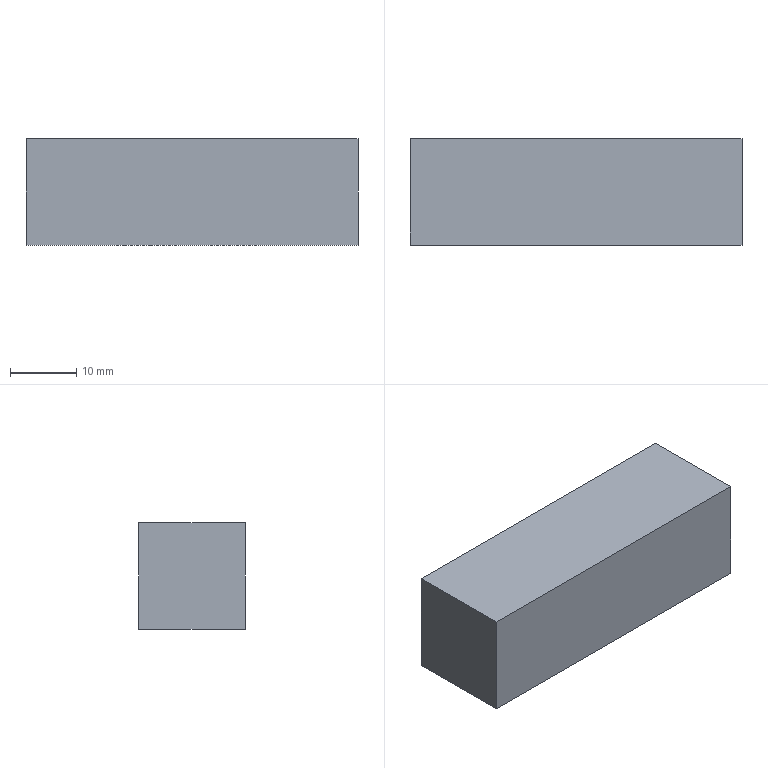Part | STEP file | [21]-1 | 1 solid | 6 faces | box 50 x 16 x 16 mm | volume 12800 mm3 | plane 6
STEP:
#1=CARTESIAN_POINT('',(0.,0.,0.));
#2=VERTEX_POINT('',#1);
#3=CARTESIAN_POINT('',(0.,16.,0.));
#4=VERTEX_POINT('',#3);
#5=CARTESIAN_POINT('',(0.,8.,0.));
#6=DIRECTION('',(0.,1.,0.));
#7=VECTOR('',#6,1000.);
#8=LINE('',#5,#7);
#9=EDGE_CURVE('',#2,#4,#8,.T.);
#10=ORIENTED_EDGE('',*,*,#9,.F.);
#11=CARTESIAN_POINT('',(0.,0.,16.));
#12=VERTEX_POINT('',#11);
#13=CARTESIAN_POINT('',(0.,0.,8.));
#14=DIRECTION('',(0.,0.,-1.));
#15=VECTOR('',#14,1000.);
#16=LINE('',#13,#15);
#17=EDGE_CURVE('',#12,#2,#16,.T.);
#18=ORIENTED_EDGE('',*,*,#17,.F.);
#19=CARTESIAN_POINT('',(0.,16.,16.));
#20=VERTEX_POINT('',#19);
#21=CARTESIAN_POINT('',(0.,8.,16.));
#22=DIRECTION('',(0.,-1.,0.));
#23=VECTOR('',#22,1000.);
#24=LINE('',#21,#23);
#25=EDGE_CURVE('',#20,#12,#24,.T.);
#26=ORIENTED_EDGE('',*,*,#25,.F.);
#27=CARTESIAN_POINT('',(0.,16.,8.));
#28=DIRECTION('',(0.,0.,1.));
#29=VECTOR('',#28,1000.);
#30=LINE('',#27,#29);
#31=EDGE_CURVE('',#4,#20,#30,.T.);
#32=ORIENTED_EDGE('',*,*,#31,.F.);
#33=EDGE_LOOP('',(#10,#18,#26,#32));
#34=FACE_OUTER_BOUND('',#33,.T.);
#35=CARTESIAN_POINT('',(0.,8.,8.));
#36=DIRECTION('',(-1.,0.,0.));
#37=DIRECTION('',(0.,-1.,0.));
#38=AXIS2_PLACEMENT_3D('',#35,#36,#37);
#39=PLANE('',#38);
#40=ADVANCED_FACE('',(#34),#39,.T.);
#41=CARTESIAN_POINT('',(50.,0.,0.));
#42=VERTEX_POINT('',#41);
#43=CARTESIAN_POINT('',(50.,0.,0.));
#44=DIRECTION('',(-1.,0.,0.));
#45=VECTOR('',#44,1000.);
#46=LINE('',#43,#45);
#47=EDGE_CURVE('',#42,#2,#46,.T.);
#48=ORIENTED_EDGE('',*,*,#47,.T.);
#49=ORIENTED_EDGE('',*,*,#9,.T.);
#50=CARTESIAN_POINT('',(50.,16.,0.));
#51=VERTEX_POINT('',#50);
#52=CARTESIAN_POINT('',(50.,16.,0.));
#53=DIRECTION('',(-1.,0.,0.));
#54=VECTOR('',#53,1000.);
#55=LINE('',#52,#54);
#56=EDGE_CURVE('',#51,#4,#55,.T.);
#57=ORIENTED_EDGE('',*,*,#56,.F.);
#58=CARTESIAN_POINT('',(50.,8.,0.));
#59=DIRECTION('',(0.,-1.,0.));
#60=VECTOR('',#59,1000.);
#61=LINE('',#58,#60);
#62=EDGE_CURVE('',#51,#42,#61,.T.);
#63=ORIENTED_EDGE('',*,*,#62,.T.);
#64=EDGE_LOOP('',(#48,#49,#57,#63));
#65=FACE_OUTER_BOUND('',#64,.T.);
#66=CARTESIAN_POINT('',(50.,8.,0.));
#67=DIRECTION('',(0.,0.,-1.));
#68=DIRECTION('',(1.,0.,0.));
#69=AXIS2_PLACEMENT_3D('',#66,#67,#68);
#70=PLANE('',#69);
#71=ADVANCED_FACE('',(#65),#70,.T.);
#72=ORIENTED_EDGE('',*,*,#56,.T.);
#73=ORIENTED_EDGE('',*,*,#31,.T.);
#74=CARTESIAN_POINT('',(50.,16.,16.));
#75=VERTEX_POINT('',#74);
#76=CARTESIAN_POINT('',(50.,16.,16.));
#77=DIRECTION('',(-1.,0.,0.));
#78=VECTOR('',#77,1000.);
#79=LINE('',#76,#78);
#80=EDGE_CURVE('',#75,#20,#79,.T.);
#81=ORIENTED_EDGE('',*,*,#80,.F.);
#82=CARTESIAN_POINT('',(50.,16.,8.));
#83=DIRECTION('',(0.,0.,-1.));
#84=VECTOR('',#83,1000.);
#85=LINE('',#82,#84);
#86=EDGE_CURVE('',#75,#51,#85,.T.);
#87=ORIENTED_EDGE('',*,*,#86,.T.);
#88=EDGE_LOOP('',(#72,#73,#81,#87));
#89=FACE_OUTER_BOUND('',#88,.T.);
#90=CARTESIAN_POINT('',(50.,16.,8.));
#91=DIRECTION('',(0.,1.,0.));
#92=DIRECTION('',(-1.,0.,0.));
#93=AXIS2_PLACEMENT_3D('',#90,#91,#92);
#94=PLANE('',#93);
#95=ADVANCED_FACE('',(#89),#94,.T.);
#96=ORIENTED_EDGE('',*,*,#80,.T.);
#97=ORIENTED_EDGE('',*,*,#25,.T.);
#98=CARTESIAN_POINT('',(50.,0.,16.));
#99=VERTEX_POINT('',#98);
#100=CARTESIAN_POINT('',(50.,0.,16.));
#101=DIRECTION('',(-1.,0.,0.));
#102=VECTOR('',#101,1000.);
#103=LINE('',#100,#102);
#104=EDGE_CURVE('',#99,#12,#103,.T.);
#105=ORIENTED_EDGE('',*,*,#104,.F.);
#106=CARTESIAN_POINT('',(50.,8.,16.));
#107=DIRECTION('',(0.,1.,0.));
#108=VECTOR('',#107,1000.);
#109=LINE('',#106,#108);
#110=EDGE_CURVE('',#99,#75,#109,.T.);
#111=ORIENTED_EDGE('',*,*,#110,.T.);
#112=EDGE_LOOP('',(#96,#97,#105,#111));
#113=FACE_OUTER_BOUND('',#112,.T.);
#114=CARTESIAN_POINT('',(50.,8.,16.));
#115=DIRECTION('',(0.,0.,1.));
#116=DIRECTION('',(-1.,0.,0.));
#117=AXIS2_PLACEMENT_3D('',#114,#115,#116);
#118=PLANE('',#117);
#119=ADVANCED_FACE('',(#113),#118,.T.);
#120=CARTESIAN_POINT('',(50.,0.,8.));
#121=DIRECTION('',(0.,0.,1.));
#122=VECTOR('',#121,1000.);
#123=LINE('',#120,#122);
#124=EDGE_CURVE('',#42,#99,#123,.T.);
#125=ORIENTED_EDGE('',*,*,#124,.F.);
#126=ORIENTED_EDGE('',*,*,#62,.F.);
#127=ORIENTED_EDGE('',*,*,#86,.F.);
#128=ORIENTED_EDGE('',*,*,#110,.F.);
#129=EDGE_LOOP('',(#125,#126,#127,#128));
#130=FACE_OUTER_BOUND('',#129,.T.);
#131=CARTESIAN_POINT('',(50.,8.,8.));
#132=DIRECTION('',(1.,0.,0.));
#133=DIRECTION('',(0.,1.,0.));
#134=AXIS2_PLACEMENT_3D('',#131,#132,#133);
#135=PLANE('',#134);
#136=ADVANCED_FACE('',(#130),#135,.T.);
#137=ORIENTED_EDGE('',*,*,#124,.T.);
#138=ORIENTED_EDGE('',*,*,#104,.T.);
#139=ORIENTED_EDGE('',*,*,#17,.T.);
#140=ORIENTED_EDGE('',*,*,#47,.F.);
#141=EDGE_LOOP('',(#137,#138,#139,#140));
#142=FACE_OUTER_BOUND('',#141,.T.);
#143=CARTESIAN_POINT('',(50.,0.,8.));
#144=DIRECTION('',(0.,-1.,0.));
#145=DIRECTION('',(1.,0.,0.));
#146=AXIS2_PLACEMENT_3D('',#143,#144,#145);
#147=PLANE('',#146);
#148=ADVANCED_FACE('',(#142),#147,.T.);
#149=CLOSED_SHELL('',(#40,#71,#95,#119,#136,#148));
#150=MANIFOLD_SOLID_BREP('',#149);
#151=CARTESIAN_POINT('',(0.,0.,0.));
#152=DIRECTION('',(0.,0.,1.));
#153=DIRECTION('',(1.,0.,0.));
#154=AXIS2_PLACEMENT_3D('',#151,#152,#153);
#155=(LENGTH_UNIT()NAMED_UNIT(*)SI_UNIT(.MILLI.,.METRE.));
#156=UNCERTAINTY_MEASURE_WITH_UNIT(LENGTH_MEASURE(0.00001),#155,'','');
#157=(NAMED_UNIT(*)PLANE_ANGLE_UNIT()SI_UNIT($,.RADIAN.));
#158=(NAMED_UNIT(*)SI_UNIT($,.STERADIAN.)SOLID_ANGLE_UNIT());
#159=(GEOMETRIC_REPRESENTATION_CONTEXT(3)GLOBAL_UNCERTAINTY_ASSIGNED_CONTEXT((#156))GLOBAL_UNIT_ASSIGNED_CONTEXT((#155,#157,#158))REPRESENTATION_CONTEXT('',''));
#160=ADVANCED_BREP_SHAPE_REPRESENTATION('',(#150,#154),#159);